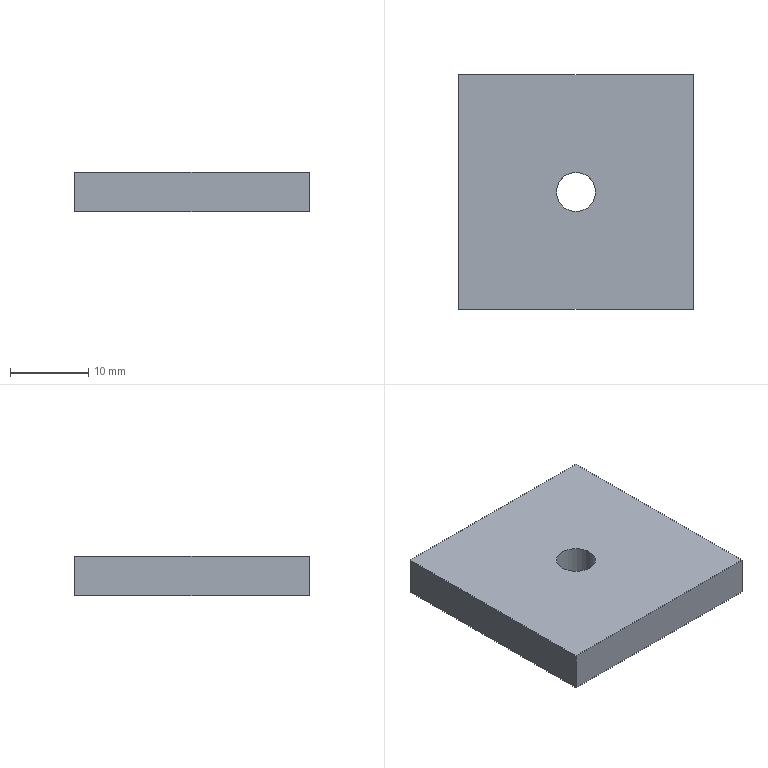Part | STEP file | Small weld block | 1 solid | 8 faces | box 30 x 30 x 5 mm | volume 4402 mm3 | plane 6 | cylinder 2 | commonest cylinder face diameters 5 x2
STEP:
#1=CARTESIAN_POINT('',(0.,0.,0.));
#2=DIRECTION('',(0.,0.,1.));
#3=DIRECTION('',(1.,0.,0.));
#4=AXIS2_PLACEMENT_3D('',#1,#2,#3);
#5=CARTESIAN_POINT('',(2.5,0.,-2.5));
#6=VERTEX_POINT('',#5);
#7=CARTESIAN_POINT('',(2.5,0.,2.5));
#8=VERTEX_POINT('',#7);
#9=CARTESIAN_POINT('',(2.5,0.,2.5));
#10=DIRECTION('',(0.,0.,1.));
#11=VECTOR('',#10,1.);
#12=LINE('',#9,#11);
#13=CARTESIAN_POINT('',(0.,0.,2.5));
#14=DIRECTION('',(0.,0.,1.));
#15=DIRECTION('',(1.,0.,0.));
#16=AXIS2_PLACEMENT_3D('',#13,#14,#15);
#17=CYLINDRICAL_SURFACE('',#16,2.5);
#18=CARTESIAN_POINT('',(6.283,0.));
#19=DIRECTION('',(0.,1.));
#20=VECTOR('',#19,1.);
#21=LINE('',#18,#20);
#22=(GEOMETRIC_REPRESENTATION_CONTEXT(2)PARAMETRIC_REPRESENTATION_CONTEXT()REPRESENTATION_CONTEXT('',''));
#23=DEFINITIONAL_REPRESENTATION('',(#21),#22);
#24=PCURVE('',#17,#23);
#25=CARTESIAN_POINT('',(0.,0.,2.5));
#26=DIRECTION('',(0.,0.,1.));
#27=DIRECTION('',(1.,0.,0.));
#28=AXIS2_PLACEMENT_3D('',#25,#26,#27);
#29=CYLINDRICAL_SURFACE('',#28,2.5);
#30=CARTESIAN_POINT('',(0.,0.));
#31=DIRECTION('',(0.,1.));
#32=VECTOR('',#31,1.);
#33=LINE('',#30,#32);
#34=(GEOMETRIC_REPRESENTATION_CONTEXT(2)PARAMETRIC_REPRESENTATION_CONTEXT()REPRESENTATION_CONTEXT('',''));
#35=DEFINITIONAL_REPRESENTATION('',(#33),#34);
#36=PCURVE('',#29,#35);
#37=SURFACE_CURVE('',#12,(#24,#36),.PCURVE_S1.);
#38=EDGE_CURVE('',#6,#8,#37,.T.);
#39=ORIENTED_EDGE('',*,*,#38,.T.);
#40=CARTESIAN_POINT('',(-2.5,0.,2.5));
#41=VERTEX_POINT('',#40);
#42=CARTESIAN_POINT('',(0.,0.,2.5));
#43=DIRECTION('',(0.,0.,1.));
#44=DIRECTION('',(1.,0.,0.));
#45=AXIS2_PLACEMENT_3D('',#42,#43,#44);
#46=CIRCLE('',#45,2.5);
#47=CARTESIAN_POINT('',(0.,0.));
#48=DIRECTION('',(1.,0.));
#49=VECTOR('',#48,1.);
#50=LINE('',#47,#49);
#51=(GEOMETRIC_REPRESENTATION_CONTEXT(2)PARAMETRIC_REPRESENTATION_CONTEXT()REPRESENTATION_CONTEXT('',''));
#52=DEFINITIONAL_REPRESENTATION('',(#50),#51);
#53=PCURVE('',#17,#52);
#54=CARTESIAN_POINT('',(0.,0.,2.5));
#55=DIRECTION('',(0.,0.,-1.));
#56=DIRECTION('',(-1.,0.,0.));
#57=AXIS2_PLACEMENT_3D('',#54,#55,#56);
#58=PLANE('',#57);
#59=CARTESIAN_POINT('',(-2.5,0.));
#60=CARTESIAN_POINT('',(-2.5,4.33));
#61=CARTESIAN_POINT('',(1.25,2.165));
#62=CARTESIAN_POINT('',(5.,0.));
#63=CARTESIAN_POINT('',(1.25,-2.165));
#64=CARTESIAN_POINT('',(-2.5,-4.33));
#65=CARTESIAN_POINT('',(-2.5,0.));
#66=(BOUNDED_CURVE()B_SPLINE_CURVE(2,(#59,#60,#61,#62,#63,#64,#65),.UNSPECIFIED.,.T.,.F.)B_SPLINE_CURVE_WITH_KNOTS((1,2,2,2,2,1),(-2.094,0.,2.094,4.189,6.283,8.378),.UNSPECIFIED.)CURVE()GEOMETRIC_REPRESENTATION_ITEM()RATIONAL_B_SPLINE_CURVE((1.,0.5,1.,0.5,1.,0.5,1.))REPRESENTATION_ITEM(''));
#67=(GEOMETRIC_REPRESENTATION_CONTEXT(2)PARAMETRIC_REPRESENTATION_CONTEXT()REPRESENTATION_CONTEXT('',''));
#68=DEFINITIONAL_REPRESENTATION('',(#66),#67);
#69=PCURVE('',#58,#68);
#70=SURFACE_CURVE('',#46,(#53,#69),.PCURVE_S1.);
#71=EDGE_CURVE('',#41,#8,#70,.T.);
#72=ORIENTED_EDGE('',*,*,#71,.F.);
#73=CARTESIAN_POINT('',(-2.5,0.,-2.5));
#74=VERTEX_POINT('',#73);
#75=CARTESIAN_POINT('',(-2.5,0.,2.5));
#76=DIRECTION('',(0.,0.,1.));
#77=VECTOR('',#76,1.);
#78=LINE('',#75,#77);
#79=CARTESIAN_POINT('',(3.142,0.));
#80=DIRECTION('',(0.,1.));
#81=VECTOR('',#80,1.);
#82=LINE('',#79,#81);
#83=(GEOMETRIC_REPRESENTATION_CONTEXT(2)PARAMETRIC_REPRESENTATION_CONTEXT()REPRESENTATION_CONTEXT('',''));
#84=DEFINITIONAL_REPRESENTATION('',(#82),#83);
#85=PCURVE('',#17,#84);
#86=CARTESIAN_POINT('',(3.142,0.));
#87=DIRECTION('',(0.,1.));
#88=VECTOR('',#87,1.);
#89=LINE('',#86,#88);
#90=(GEOMETRIC_REPRESENTATION_CONTEXT(2)PARAMETRIC_REPRESENTATION_CONTEXT()REPRESENTATION_CONTEXT('',''));
#91=DEFINITIONAL_REPRESENTATION('',(#89),#90);
#92=PCURVE('',#29,#91);
#93=SURFACE_CURVE('',#78,(#85,#92),.PCURVE_S1.);
#94=EDGE_CURVE('',#74,#41,#93,.T.);
#95=ORIENTED_EDGE('',*,*,#94,.F.);
#96=CARTESIAN_POINT('',(0.,0.,-2.5));
#97=DIRECTION('',(0.,0.,1.));
#98=DIRECTION('',(1.,0.,0.));
#99=AXIS2_PLACEMENT_3D('',#96,#97,#98);
#100=CIRCLE('',#99,2.5);
#101=CARTESIAN_POINT('',(0.,-5.));
#102=DIRECTION('',(1.,0.));
#103=VECTOR('',#102,1.);
#104=LINE('',#101,#103);
#105=(GEOMETRIC_REPRESENTATION_CONTEXT(2)PARAMETRIC_REPRESENTATION_CONTEXT()REPRESENTATION_CONTEXT('',''));
#106=DEFINITIONAL_REPRESENTATION('',(#104),#105);
#107=PCURVE('',#17,#106);
#108=CARTESIAN_POINT('',(0.,0.,-2.5));
#109=DIRECTION('',(0.,0.,-1.));
#110=DIRECTION('',(-1.,0.,0.));
#111=AXIS2_PLACEMENT_3D('',#108,#109,#110);
#112=PLANE('',#111);
#113=CARTESIAN_POINT('',(-2.5,0.));
#114=CARTESIAN_POINT('',(-2.5,4.33));
#115=CARTESIAN_POINT('',(1.25,2.165));
#116=CARTESIAN_POINT('',(5.,0.));
#117=CARTESIAN_POINT('',(1.25,-2.165));
#118=CARTESIAN_POINT('',(-2.5,-4.33));
#119=CARTESIAN_POINT('',(-2.5,0.));
#120=(BOUNDED_CURVE()B_SPLINE_CURVE(2,(#113,#114,#115,#116,#117,#118,#119),.UNSPECIFIED.,.T.,.F.)B_SPLINE_CURVE_WITH_KNOTS((1,2,2,2,2,1),(-2.094,0.,2.094,4.189,6.283,8.378),.UNSPECIFIED.)CURVE()GEOMETRIC_REPRESENTATION_ITEM()RATIONAL_B_SPLINE_CURVE((1.,0.5,1.,0.5,1.,0.5,1.))REPRESENTATION_ITEM(''));
#121=(GEOMETRIC_REPRESENTATION_CONTEXT(2)PARAMETRIC_REPRESENTATION_CONTEXT()REPRESENTATION_CONTEXT('',''));
#122=DEFINITIONAL_REPRESENTATION('',(#120),#121);
#123=PCURVE('',#112,#122);
#124=SURFACE_CURVE('',#100,(#107,#123),.PCURVE_S1.);
#125=EDGE_CURVE('',#74,#6,#124,.T.);
#126=ORIENTED_EDGE('',*,*,#125,.T.);
#127=EDGE_LOOP('',(#39,#72,#95,#126));
#128=FACE_BOUND('',#127,.F.);
#129=ADVANCED_FACE('',(#128),#17,.F.);
#130=CARTESIAN_POINT('',(15.,-15.,-2.5));
#131=VERTEX_POINT('',#130);
#132=CARTESIAN_POINT('',(15.,15.,-2.5));
#133=VERTEX_POINT('',#132);
#134=CARTESIAN_POINT('',(15.,-15.,-2.5));
#135=DIRECTION('',(0.,1.,0.));
#136=VECTOR('',#135,1.);
#137=LINE('',#134,#136);
#138=CARTESIAN_POINT('',(15.,-15.,2.5));
#139=DIRECTION('',(-1.,0.,0.));
#140=DIRECTION('',(0.,0.,1.));
#141=AXIS2_PLACEMENT_3D('',#138,#139,#140);
#142=PLANE('',#141);
#143=CARTESIAN_POINT('',(-5.,0.));
#144=DIRECTION('',(0.,1.));
#145=VECTOR('',#144,1.);
#146=LINE('',#143,#145);
#147=(GEOMETRIC_REPRESENTATION_CONTEXT(2)PARAMETRIC_REPRESENTATION_CONTEXT()REPRESENTATION_CONTEXT('',''));
#148=DEFINITIONAL_REPRESENTATION('',(#146),#147);
#149=PCURVE('',#142,#148);
#150=CARTESIAN_POINT('',(-15.,-15.));
#151=DIRECTION('',(0.,1.));
#152=VECTOR('',#151,1.);
#153=LINE('',#150,#152);
#154=(GEOMETRIC_REPRESENTATION_CONTEXT(2)PARAMETRIC_REPRESENTATION_CONTEXT()REPRESENTATION_CONTEXT('',''));
#155=DEFINITIONAL_REPRESENTATION('',(#153),#154);
#156=PCURVE('',#112,#155);
#157=SURFACE_CURVE('',#137,(#149,#156),.PCURVE_S1.);
#158=EDGE_CURVE('',#131,#133,#157,.T.);
#159=ORIENTED_EDGE('',*,*,#158,.T.);
#160=CARTESIAN_POINT('',(15.,15.,2.5));
#161=VERTEX_POINT('',#160);
#162=CARTESIAN_POINT('',(15.,15.,2.5));
#163=DIRECTION('',(0.,0.,-1.));
#164=VECTOR('',#163,1.);
#165=LINE('',#162,#164);
#166=CARTESIAN_POINT('',(0.,30.));
#167=DIRECTION('',(-1.,0.));
#168=VECTOR('',#167,1.);
#169=LINE('',#166,#168);
#170=(GEOMETRIC_REPRESENTATION_CONTEXT(2)PARAMETRIC_REPRESENTATION_CONTEXT()REPRESENTATION_CONTEXT('',''));
#171=DEFINITIONAL_REPRESENTATION('',(#169),#170);
#172=PCURVE('',#142,#171);
#173=CARTESIAN_POINT('',(-15.,15.,2.5));
#174=DIRECTION('',(0.,-1.,0.));
#175=DIRECTION('',(0.,0.,-1.));
#176=AXIS2_PLACEMENT_3D('',#173,#174,#175);
#177=PLANE('',#176);
#178=CARTESIAN_POINT('',(0.,30.));
#179=DIRECTION('',(1.,0.));
#180=VECTOR('',#179,1.);
#181=LINE('',#178,#180);
#182=(GEOMETRIC_REPRESENTATION_CONTEXT(2)PARAMETRIC_REPRESENTATION_CONTEXT()REPRESENTATION_CONTEXT('',''));
#183=DEFINITIONAL_REPRESENTATION('',(#181),#182);
#184=PCURVE('',#177,#183);
#185=SURFACE_CURVE('',#165,(#172,#184),.PCURVE_S1.);
#186=EDGE_CURVE('',#161,#133,#185,.T.);
#187=ORIENTED_EDGE('',*,*,#186,.F.);
#188=CARTESIAN_POINT('',(15.,-15.,2.5));
#189=VERTEX_POINT('',#188);
#190=CARTESIAN_POINT('',(15.,-15.,2.5));
#191=DIRECTION('',(0.,1.,0.));
#192=VECTOR('',#191,1.);
#193=LINE('',#190,#192);
#194=CARTESIAN_POINT('',(0.,0.));
#195=DIRECTION('',(0.,1.));
#196=VECTOR('',#195,1.);
#197=LINE('',#194,#196);
#198=(GEOMETRIC_REPRESENTATION_CONTEXT(2)PARAMETRIC_REPRESENTATION_CONTEXT()REPRESENTATION_CONTEXT('',''));
#199=DEFINITIONAL_REPRESENTATION('',(#197),#198);
#200=PCURVE('',#142,#199);
#201=CARTESIAN_POINT('',(-15.,-15.));
#202=DIRECTION('',(0.,1.));
#203=VECTOR('',#202,1.);
#204=LINE('',#201,#203);
#205=(GEOMETRIC_REPRESENTATION_CONTEXT(2)PARAMETRIC_REPRESENTATION_CONTEXT()REPRESENTATION_CONTEXT('',''));
#206=DEFINITIONAL_REPRESENTATION('',(#204),#205);
#207=PCURVE('',#58,#206);
#208=SURFACE_CURVE('',#193,(#200,#207),.PCURVE_S1.);
#209=EDGE_CURVE('',#189,#161,#208,.T.);
#210=ORIENTED_EDGE('',*,*,#209,.F.);
#211=CARTESIAN_POINT('',(15.,-15.,2.5));
#212=DIRECTION('',(0.,0.,-1.));
#213=VECTOR('',#212,1.);
#214=LINE('',#211,#213);
#215=CARTESIAN_POINT('',(0.,0.));
#216=DIRECTION('',(-1.,0.));
#217=VECTOR('',#216,1.);
#218=LINE('',#215,#217);
#219=(GEOMETRIC_REPRESENTATION_CONTEXT(2)PARAMETRIC_REPRESENTATION_CONTEXT()REPRESENTATION_CONTEXT('',''));
#220=DEFINITIONAL_REPRESENTATION('',(#218),#219);
#221=PCURVE('',#142,#220);
#222=CARTESIAN_POINT('',(-15.,-15.,2.5));
#223=DIRECTION('',(0.,1.,0.));
#224=DIRECTION('',(0.,0.,1.));
#225=AXIS2_PLACEMENT_3D('',#222,#223,#224);
#226=PLANE('',#225);
#227=CARTESIAN_POINT('',(0.,30.));
#228=DIRECTION('',(-1.,0.));
#229=VECTOR('',#228,1.);
#230=LINE('',#227,#229);
#231=(GEOMETRIC_REPRESENTATION_CONTEXT(2)PARAMETRIC_REPRESENTATION_CONTEXT()REPRESENTATION_CONTEXT('',''));
#232=DEFINITIONAL_REPRESENTATION('',(#230),#231);
#233=PCURVE('',#226,#232);
#234=SURFACE_CURVE('',#214,(#221,#233),.PCURVE_S1.);
#235=EDGE_CURVE('',#189,#131,#234,.T.);
#236=ORIENTED_EDGE('',*,*,#235,.T.);
#237=EDGE_LOOP('',(#159,#187,#210,#236));
#238=FACE_BOUND('',#237,.T.);
#239=ADVANCED_FACE('',(#238),#142,.F.);
#240=CARTESIAN_POINT('',(-15.,15.,-2.5));
#241=VERTEX_POINT('',#240);
#242=CARTESIAN_POINT('',(-15.,15.,-2.5));
#243=DIRECTION('',(-1.,0.,0.));
#244=VECTOR('',#243,1.);
#245=LINE('',#242,#244);
#246=CARTESIAN_POINT('',(5.,0.));
#247=DIRECTION('',(0.,-1.));
#248=VECTOR('',#247,1.);
#249=LINE('',#246,#248);
#250=(GEOMETRIC_REPRESENTATION_CONTEXT(2)PARAMETRIC_REPRESENTATION_CONTEXT()REPRESENTATION_CONTEXT('',''));
#251=DEFINITIONAL_REPRESENTATION('',(#249),#250);
#252=PCURVE('',#177,#251);
#253=CARTESIAN_POINT('',(15.,15.));
#254=DIRECTION('',(1.,0.));
#255=VECTOR('',#254,1.);
#256=LINE('',#253,#255);
#257=(GEOMETRIC_REPRESENTATION_CONTEXT(2)PARAMETRIC_REPRESENTATION_CONTEXT()REPRESENTATION_CONTEXT('',''));
#258=DEFINITIONAL_REPRESENTATION('',(#256),#257);
#259=PCURVE('',#112,#258);
#260=SURFACE_CURVE('',#245,(#252,#259),.PCURVE_S1.);
#261=EDGE_CURVE('',#133,#241,#260,.T.);
#262=ORIENTED_EDGE('',*,*,#261,.T.);
#263=CARTESIAN_POINT('',(-15.,15.,2.5));
#264=VERTEX_POINT('',#263);
#265=CARTESIAN_POINT('',(-15.,15.,2.5));
#266=DIRECTION('',(0.,0.,-1.));
#267=VECTOR('',#266,1.);
#268=LINE('',#265,#267);
#269=CARTESIAN_POINT('',(0.,0.));
#270=DIRECTION('',(1.,0.));
#271=VECTOR('',#270,1.);
#272=LINE('',#269,#271);
#273=(GEOMETRIC_REPRESENTATION_CONTEXT(2)PARAMETRIC_REPRESENTATION_CONTEXT()REPRESENTATION_CONTEXT('',''));
#274=DEFINITIONAL_REPRESENTATION('',(#272),#273);
#275=PCURVE('',#177,#274);
#276=CARTESIAN_POINT('',(-15.,-15.,2.5));
#277=DIRECTION('',(1.,0.,0.));
#278=DIRECTION('',(0.,0.,-1.));
#279=AXIS2_PLACEMENT_3D('',#276,#277,#278);
#280=PLANE('',#279);
#281=CARTESIAN_POINT('',(0.,30.));
#282=DIRECTION('',(1.,0.));
#283=VECTOR('',#282,1.);
#284=LINE('',#281,#283);
#285=(GEOMETRIC_REPRESENTATION_CONTEXT(2)PARAMETRIC_REPRESENTATION_CONTEXT()REPRESENTATION_CONTEXT('',''));
#286=DEFINITIONAL_REPRESENTATION('',(#284),#285);
#287=PCURVE('',#280,#286);
#288=SURFACE_CURVE('',#268,(#275,#287),.PCURVE_S1.);
#289=EDGE_CURVE('',#264,#241,#288,.T.);
#290=ORIENTED_EDGE('',*,*,#289,.F.);
#291=CARTESIAN_POINT('',(-15.,15.,2.5));
#292=DIRECTION('',(-1.,0.,0.));
#293=VECTOR('',#292,1.);
#294=LINE('',#291,#293);
#295=CARTESIAN_POINT('',(0.,0.));
#296=DIRECTION('',(0.,-1.));
#297=VECTOR('',#296,1.);
#298=LINE('',#295,#297);
#299=(GEOMETRIC_REPRESENTATION_CONTEXT(2)PARAMETRIC_REPRESENTATION_CONTEXT()REPRESENTATION_CONTEXT('',''));
#300=DEFINITIONAL_REPRESENTATION('',(#298),#299);
#301=PCURVE('',#177,#300);
#302=CARTESIAN_POINT('',(15.,15.));
#303=DIRECTION('',(1.,0.));
#304=VECTOR('',#303,1.);
#305=LINE('',#302,#304);
#306=(GEOMETRIC_REPRESENTATION_CONTEXT(2)PARAMETRIC_REPRESENTATION_CONTEXT()REPRESENTATION_CONTEXT('',''));
#307=DEFINITIONAL_REPRESENTATION('',(#305),#306);
#308=PCURVE('',#58,#307);
#309=SURFACE_CURVE('',#294,(#301,#308),.PCURVE_S1.);
#310=EDGE_CURVE('',#161,#264,#309,.T.);
#311=ORIENTED_EDGE('',*,*,#310,.F.);
#312=ORIENTED_EDGE('',*,*,#186,.T.);
#313=EDGE_LOOP('',(#262,#290,#311,#312));
#314=FACE_BOUND('',#313,.T.);
#315=ADVANCED_FACE('',(#314),#177,.F.);
#316=CARTESIAN_POINT('',(-15.,-15.,-2.5));
#317=VERTEX_POINT('',#316);
#318=CARTESIAN_POINT('',(-15.,-15.,-2.5));
#319=DIRECTION('',(0.,-1.,0.));
#320=VECTOR('',#319,1.);
#321=LINE('',#318,#320);
#322=CARTESIAN_POINT('',(5.,0.));
#323=DIRECTION('',(0.,-1.));
#324=VECTOR('',#323,1.);
#325=LINE('',#322,#324);
#326=(GEOMETRIC_REPRESENTATION_CONTEXT(2)PARAMETRIC_REPRESENTATION_CONTEXT()REPRESENTATION_CONTEXT('',''));
#327=DEFINITIONAL_REPRESENTATION('',(#325),#326);
#328=PCURVE('',#280,#327);
#329=CARTESIAN_POINT('',(15.,-15.));
#330=DIRECTION('',(0.,-1.));
#331=VECTOR('',#330,1.);
#332=LINE('',#329,#331);
#333=(GEOMETRIC_REPRESENTATION_CONTEXT(2)PARAMETRIC_REPRESENTATION_CONTEXT()REPRESENTATION_CONTEXT('',''));
#334=DEFINITIONAL_REPRESENTATION('',(#332),#333);
#335=PCURVE('',#112,#334);
#336=SURFACE_CURVE('',#321,(#328,#335),.PCURVE_S1.);
#337=EDGE_CURVE('',#241,#317,#336,.T.);
#338=ORIENTED_EDGE('',*,*,#337,.T.);
#339=CARTESIAN_POINT('',(-15.,-15.,2.5));
#340=VERTEX_POINT('',#339);
#341=CARTESIAN_POINT('',(-15.,-15.,2.5));
#342=DIRECTION('',(0.,0.,-1.));
#343=VECTOR('',#342,1.);
#344=LINE('',#341,#343);
#345=CARTESIAN_POINT('',(0.,0.));
#346=DIRECTION('',(1.,0.));
#347=VECTOR('',#346,1.);
#348=LINE('',#345,#347);
#349=(GEOMETRIC_REPRESENTATION_CONTEXT(2)PARAMETRIC_REPRESENTATION_CONTEXT()REPRESENTATION_CONTEXT('',''));
#350=DEFINITIONAL_REPRESENTATION('',(#348),#349);
#351=PCURVE('',#280,#350);
#352=CARTESIAN_POINT('',(0.,0.));
#353=DIRECTION('',(-1.,0.));
#354=VECTOR('',#353,1.);
#355=LINE('',#352,#354);
#356=(GEOMETRIC_REPRESENTATION_CONTEXT(2)PARAMETRIC_REPRESENTATION_CONTEXT()REPRESENTATION_CONTEXT('',''));
#357=DEFINITIONAL_REPRESENTATION('',(#355),#356);
#358=PCURVE('',#226,#357);
#359=SURFACE_CURVE('',#344,(#351,#358),.PCURVE_S1.);
#360=EDGE_CURVE('',#340,#317,#359,.T.);
#361=ORIENTED_EDGE('',*,*,#360,.F.);
#362=CARTESIAN_POINT('',(-15.,-15.,2.5));
#363=DIRECTION('',(0.,-1.,0.));
#364=VECTOR('',#363,1.);
#365=LINE('',#362,#364);
#366=CARTESIAN_POINT('',(0.,0.));
#367=DIRECTION('',(0.,-1.));
#368=VECTOR('',#367,1.);
#369=LINE('',#366,#368);
#370=(GEOMETRIC_REPRESENTATION_CONTEXT(2)PARAMETRIC_REPRESENTATION_CONTEXT()REPRESENTATION_CONTEXT('',''));
#371=DEFINITIONAL_REPRESENTATION('',(#369),#370);
#372=PCURVE('',#280,#371);
#373=CARTESIAN_POINT('',(15.,-15.));
#374=DIRECTION('',(0.,-1.));
#375=VECTOR('',#374,1.);
#376=LINE('',#373,#375);
#377=(GEOMETRIC_REPRESENTATION_CONTEXT(2)PARAMETRIC_REPRESENTATION_CONTEXT()REPRESENTATION_CONTEXT('',''));
#378=DEFINITIONAL_REPRESENTATION('',(#376),#377);
#379=PCURVE('',#58,#378);
#380=SURFACE_CURVE('',#365,(#372,#379),.PCURVE_S1.);
#381=EDGE_CURVE('',#264,#340,#380,.T.);
#382=ORIENTED_EDGE('',*,*,#381,.F.);
#383=ORIENTED_EDGE('',*,*,#289,.T.);
#384=EDGE_LOOP('',(#338,#361,#382,#383));
#385=FACE_BOUND('',#384,.T.);
#386=ADVANCED_FACE('',(#385),#280,.F.);
#387=CARTESIAN_POINT('',(-15.,-15.,-2.5));
#388=DIRECTION('',(1.,0.,0.));
#389=VECTOR('',#388,1.);
#390=LINE('',#387,#389);
#391=CARTESIAN_POINT('',(-5.,0.));
#392=DIRECTION('',(0.,1.));
#393=VECTOR('',#392,1.);
#394=LINE('',#391,#393);
#395=(GEOMETRIC_REPRESENTATION_CONTEXT(2)PARAMETRIC_REPRESENTATION_CONTEXT()REPRESENTATION_CONTEXT('',''));
#396=DEFINITIONAL_REPRESENTATION('',(#394),#395);
#397=PCURVE('',#226,#396);
#398=CARTESIAN_POINT('',(15.,-15.));
#399=DIRECTION('',(-1.,0.));
#400=VECTOR('',#399,1.);
#401=LINE('',#398,#400);
#402=(GEOMETRIC_REPRESENTATION_CONTEXT(2)PARAMETRIC_REPRESENTATION_CONTEXT()REPRESENTATION_CONTEXT('',''));
#403=DEFINITIONAL_REPRESENTATION('',(#401),#402);
#404=PCURVE('',#112,#403);
#405=SURFACE_CURVE('',#390,(#397,#404),.PCURVE_S1.);
#406=EDGE_CURVE('',#317,#131,#405,.T.);
#407=ORIENTED_EDGE('',*,*,#406,.T.);
#408=ORIENTED_EDGE('',*,*,#235,.F.);
#409=CARTESIAN_POINT('',(-15.,-15.,2.5));
#410=DIRECTION('',(1.,0.,0.));
#411=VECTOR('',#410,1.);
#412=LINE('',#409,#411);
#413=CARTESIAN_POINT('',(0.,0.));
#414=DIRECTION('',(0.,1.));
#415=VECTOR('',#414,1.);
#416=LINE('',#413,#415);
#417=(GEOMETRIC_REPRESENTATION_CONTEXT(2)PARAMETRIC_REPRESENTATION_CONTEXT()REPRESENTATION_CONTEXT('',''));
#418=DEFINITIONAL_REPRESENTATION('',(#416),#417);
#419=PCURVE('',#226,#418);
#420=CARTESIAN_POINT('',(15.,-15.));
#421=DIRECTION('',(-1.,0.));
#422=VECTOR('',#421,1.);
#423=LINE('',#420,#422);
#424=(GEOMETRIC_REPRESENTATION_CONTEXT(2)PARAMETRIC_REPRESENTATION_CONTEXT()REPRESENTATION_CONTEXT('',''));
#425=DEFINITIONAL_REPRESENTATION('',(#423),#424);
#426=PCURVE('',#58,#425);
#427=SURFACE_CURVE('',#412,(#419,#426),.PCURVE_S1.);
#428=EDGE_CURVE('',#340,#189,#427,.T.);
#429=ORIENTED_EDGE('',*,*,#428,.F.);
#430=ORIENTED_EDGE('',*,*,#360,.T.);
#431=EDGE_LOOP('',(#407,#408,#429,#430));
#432=FACE_BOUND('',#431,.T.);
#433=ADVANCED_FACE('',(#432),#226,.F.);
#434=CARTESIAN_POINT('',(0.,0.,2.5));
#435=DIRECTION('',(0.,0.,1.));
#436=DIRECTION('',(1.,0.,0.));
#437=AXIS2_PLACEMENT_3D('',#434,#435,#436);
#438=CIRCLE('',#437,2.5);
#439=CARTESIAN_POINT('',(-2.5,0.));
#440=CARTESIAN_POINT('',(-2.5,4.33));
#441=CARTESIAN_POINT('',(1.25,2.165));
#442=CARTESIAN_POINT('',(5.,0.));
#443=CARTESIAN_POINT('',(1.25,-2.165));
#444=CARTESIAN_POINT('',(-2.5,-4.33));
#445=CARTESIAN_POINT('',(-2.5,0.));
#446=(BOUNDED_CURVE()B_SPLINE_CURVE(2,(#439,#440,#441,#442,#443,#444,#445),.UNSPECIFIED.,.T.,.F.)B_SPLINE_CURVE_WITH_KNOTS((1,2,2,2,2,1),(-2.094,0.,2.094,4.189,6.283,8.378),.UNSPECIFIED.)CURVE()GEOMETRIC_REPRESENTATION_ITEM()RATIONAL_B_SPLINE_CURVE((1.,0.5,1.,0.5,1.,0.5,1.))REPRESENTATION_ITEM(''));
#447=(GEOMETRIC_REPRESENTATION_CONTEXT(2)PARAMETRIC_REPRESENTATION_CONTEXT()REPRESENTATION_CONTEXT('',''));
#448=DEFINITIONAL_REPRESENTATION('',(#446),#447);
#449=PCURVE('',#58,#448);
#450=CARTESIAN_POINT('',(0.,0.));
#451=DIRECTION('',(1.,0.));
#452=VECTOR('',#451,1.);
#453=LINE('',#450,#452);
#454=(GEOMETRIC_REPRESENTATION_CONTEXT(2)PARAMETRIC_REPRESENTATION_CONTEXT()REPRESENTATION_CONTEXT('',''));
#455=DEFINITIONAL_REPRESENTATION('',(#453),#454);
#456=PCURVE('',#29,#455);
#457=SURFACE_CURVE('',#438,(#449,#456),.PCURVE_S1.);
#458=EDGE_CURVE('',#8,#41,#457,.T.);
#459=ORIENTED_EDGE('',*,*,#458,.F.);
#460=ORIENTED_EDGE('',*,*,#71,.F.);
#461=EDGE_LOOP('',(#459,#460));
#462=FACE_BOUND('',#461,.T.);
#463=ORIENTED_EDGE('',*,*,#209,.T.);
#464=ORIENTED_EDGE('',*,*,#310,.T.);
#465=ORIENTED_EDGE('',*,*,#381,.T.);
#466=ORIENTED_EDGE('',*,*,#428,.T.);
#467=EDGE_LOOP('',(#463,#464,#465,#466));
#468=FACE_BOUND('',#467,.T.);
#469=ADVANCED_FACE('',(#462,#468),#58,.F.);
#470=CARTESIAN_POINT('',(0.,0.,-2.5));
#471=DIRECTION('',(0.,0.,1.));
#472=DIRECTION('',(1.,0.,0.));
#473=AXIS2_PLACEMENT_3D('',#470,#471,#472);
#474=CIRCLE('',#473,2.5);
#475=CARTESIAN_POINT('',(-2.5,0.));
#476=CARTESIAN_POINT('',(-2.5,4.33));
#477=CARTESIAN_POINT('',(1.25,2.165));
#478=CARTESIAN_POINT('',(5.,0.));
#479=CARTESIAN_POINT('',(1.25,-2.165));
#480=CARTESIAN_POINT('',(-2.5,-4.33));
#481=CARTESIAN_POINT('',(-2.5,0.));
#482=(BOUNDED_CURVE()B_SPLINE_CURVE(2,(#475,#476,#477,#478,#479,#480,#481),.UNSPECIFIED.,.T.,.F.)B_SPLINE_CURVE_WITH_KNOTS((1,2,2,2,2,1),(-2.094,0.,2.094,4.189,6.283,8.378),.UNSPECIFIED.)CURVE()GEOMETRIC_REPRESENTATION_ITEM()RATIONAL_B_SPLINE_CURVE((1.,0.5,1.,0.5,1.,0.5,1.))REPRESENTATION_ITEM(''));
#483=(GEOMETRIC_REPRESENTATION_CONTEXT(2)PARAMETRIC_REPRESENTATION_CONTEXT()REPRESENTATION_CONTEXT('',''));
#484=DEFINITIONAL_REPRESENTATION('',(#482),#483);
#485=PCURVE('',#112,#484);
#486=CARTESIAN_POINT('',(0.,-5.));
#487=DIRECTION('',(1.,0.));
#488=VECTOR('',#487,1.);
#489=LINE('',#486,#488);
#490=(GEOMETRIC_REPRESENTATION_CONTEXT(2)PARAMETRIC_REPRESENTATION_CONTEXT()REPRESENTATION_CONTEXT('',''));
#491=DEFINITIONAL_REPRESENTATION('',(#489),#490);
#492=PCURVE('',#29,#491);
#493=SURFACE_CURVE('',#474,(#485,#492),.PCURVE_S1.);
#494=EDGE_CURVE('',#6,#74,#493,.T.);
#495=ORIENTED_EDGE('',*,*,#494,.T.);
#496=ORIENTED_EDGE('',*,*,#125,.T.);
#497=EDGE_LOOP('',(#495,#496));
#498=FACE_BOUND('',#497,.T.);
#499=ORIENTED_EDGE('',*,*,#158,.F.);
#500=ORIENTED_EDGE('',*,*,#406,.F.);
#501=ORIENTED_EDGE('',*,*,#337,.F.);
#502=ORIENTED_EDGE('',*,*,#261,.F.);
#503=EDGE_LOOP('',(#499,#500,#501,#502));
#504=FACE_BOUND('',#503,.T.);
#505=ADVANCED_FACE('',(#498,#504),#112,.T.);
#506=ORIENTED_EDGE('',*,*,#458,.F.);
#507=ORIENTED_EDGE('',*,*,#38,.F.);
#508=ORIENTED_EDGE('',*,*,#494,.T.);
#509=ORIENTED_EDGE('',*,*,#94,.T.);
#510=EDGE_LOOP('',(#506,#507,#508,#509));
#511=FACE_BOUND('',#510,.F.);
#512=ADVANCED_FACE('',(#511),#29,.F.);
#513=CLOSED_SHELL('',(#129,#239,#315,#386,#433,#469,#505,#512));
#514=MANIFOLD_SOLID_BREP('',#513);
#515=(LENGTH_UNIT()NAMED_UNIT(*)SI_UNIT(.MILLI.,.METRE.));
#516=UNCERTAINTY_MEASURE_WITH_UNIT(LENGTH_MEASURE(0.0000001),#515,'','');
#517=(NAMED_UNIT(*)PLANE_ANGLE_UNIT()SI_UNIT($,.RADIAN.));
#518=(NAMED_UNIT(*)SI_UNIT($,.STERADIAN.)SOLID_ANGLE_UNIT());
#519=(GEOMETRIC_REPRESENTATION_CONTEXT(3)GLOBAL_UNCERTAINTY_ASSIGNED_CONTEXT((#516))GLOBAL_UNIT_ASSIGNED_CONTEXT((#515,#517,#518))REPRESENTATION_CONTEXT('',''));
#520=ADVANCED_BREP_SHAPE_REPRESENTATION('',(#4,#514),#519);